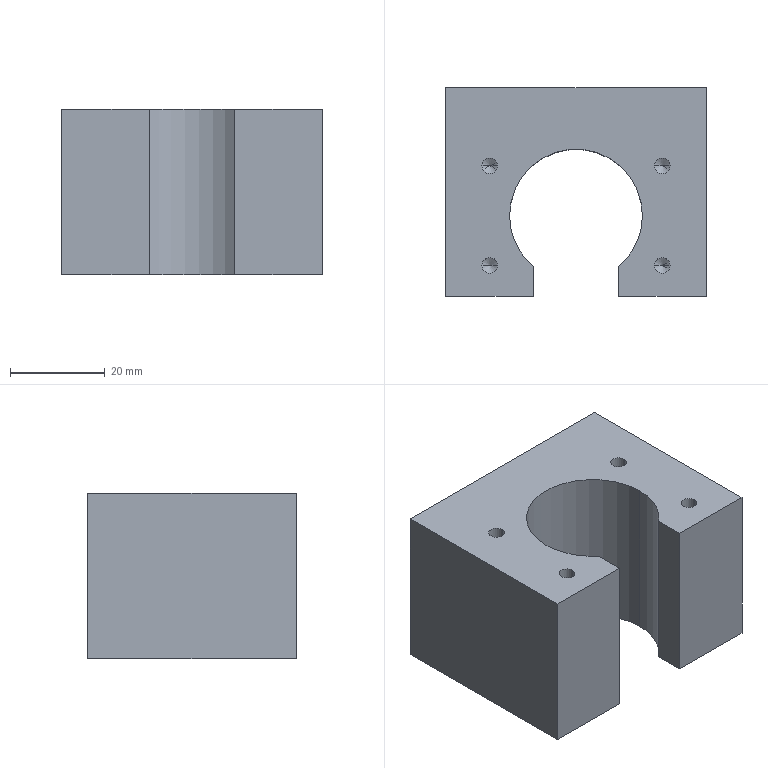Part | SolidWorks | features HoleWzd 2, 3DProfileFeature 1, Extrusion 1 | 1 solid | 52 faces | box 55 x 44 x 35 mm | volume 59279 mm3 | cone 24 | cylinder 19 | plane 9 | commonest cylinder face diameters 3.3 x8 5 x8 28 x3
STEP:
#1=CARTESIAN_POINT('',(-20.5,26.475,8.));
#2=VERTEX_POINT('',#1);
#3=CARTESIAN_POINT('',(-20.5,26.475,13.));
#4=VERTEX_POINT('',#3);
#5=CARTESIAN_POINT('',(-20.5,26.475,10.5));
#6=DIRECTION('',(0.,1.,0.));
#7=DIRECTION('',(0.,0.,1.));
#8=AXIS2_PLACEMENT_3D('',#5,#6,#7);
#9=CIRCLE('',#8,2.5);
#10=EDGE_CURVE('',#2,#4,#9,.T.);
#11=ORIENTED_EDGE('',*,*,#10,.F.);
#12=CARTESIAN_POINT('',(-20.5,27.,7.475));
#13=VERTEX_POINT('',#12);
#14=CARTESIAN_POINT('',(-20.5,27.,7.475));
#15=DIRECTION('',(0.,0.7071,-0.7071));
#16=VECTOR('',#15,1000.);
#17=LINE('',#14,#16);
#18=EDGE_CURVE('',#2,#13,#17,.T.);
#19=ORIENTED_EDGE('',*,*,#18,.T.);
#20=CARTESIAN_POINT('',(-20.5,27.,13.525));
#21=VERTEX_POINT('',#20);
#22=CARTESIAN_POINT('',(-20.5,27.,10.5));
#23=DIRECTION('',(0.,1.,0.));
#24=DIRECTION('',(0.,0.,1.));
#25=AXIS2_PLACEMENT_3D('',#22,#23,#24);
#26=CIRCLE('',#25,3.025);
#27=EDGE_CURVE('',#13,#21,#26,.T.);
#28=ORIENTED_EDGE('',*,*,#27,.T.);
#29=CARTESIAN_POINT('',(-20.5,27.,13.525));
#30=DIRECTION('',(0.,0.7071,0.7071));
#31=VECTOR('',#30,1000.);
#32=LINE('',#29,#31);
#33=EDGE_CURVE('',#4,#21,#32,.T.);
#34=ORIENTED_EDGE('',*,*,#33,.F.);
#35=EDGE_LOOP('',(#11,#19,#28,#34));
#36=FACE_OUTER_BOUND('',#35,.T.);
#37=CARTESIAN_POINT('',(-20.5,27.,10.5));
#38=DIRECTION('',(0.,1.,0.));
#39=DIRECTION('',(0.,0.,1.));
#40=AXIS2_PLACEMENT_3D('',#37,#38,#39);
#41=CONICAL_SURFACE('',#40,3.025,0.7854);
#42=ADVANCED_FACE('',(#36),#41,.F.);
#43=CARTESIAN_POINT('',(-20.5,15.,8.));
#44=VERTEX_POINT('',#43);
#45=CARTESIAN_POINT('',(-20.5,15.,13.));
#46=VERTEX_POINT('',#45);
#47=CARTESIAN_POINT('',(-20.5,15.,10.5));
#48=DIRECTION('',(0.,1.,0.));
#49=DIRECTION('',(0.,0.,1.));
#50=AXIS2_PLACEMENT_3D('',#47,#48,#49);
#51=CIRCLE('',#50,2.5);
#52=EDGE_CURVE('',#44,#46,#51,.T.);
#53=ORIENTED_EDGE('',*,*,#52,.F.);
#54=CARTESIAN_POINT('',(-20.5,27.,8.));
#55=DIRECTION('',(0.,1.,0.));
#56=VECTOR('',#55,1000.);
#57=LINE('',#54,#56);
#58=EDGE_CURVE('',#44,#2,#57,.T.);
#59=ORIENTED_EDGE('',*,*,#58,.T.);
#60=ORIENTED_EDGE('',*,*,#10,.T.);
#61=CARTESIAN_POINT('',(-20.5,27.,13.));
#62=DIRECTION('',(0.,1.,0.));
#63=VECTOR('',#62,1000.);
#64=LINE('',#61,#63);
#65=EDGE_CURVE('',#46,#4,#64,.T.);
#66=ORIENTED_EDGE('',*,*,#65,.F.);
#67=EDGE_LOOP('',(#53,#59,#60,#66));
#68=FACE_OUTER_BOUND('',#67,.T.);
#69=CARTESIAN_POINT('',(-20.5,27.,10.5));
#70=DIRECTION('',(0.,1.,0.));
#71=DIRECTION('',(0.,0.,1.));
#72=AXIS2_PLACEMENT_3D('',#69,#70,#71);
#73=CYLINDRICAL_SURFACE('',#72,2.5);
#74=ADVANCED_FACE('',(#68),#73,.F.);
#75=CARTESIAN_POINT('',(-20.5,13.498,10.5));
#76=VERTEX_POINT('',#75);
#77=CARTESIAN_POINT('',(-20.5,15.,13.));
#78=DIRECTION('',(0.,0.515,0.8572));
#79=VECTOR('',#78,1000.);
#80=LINE('',#77,#79);
#81=EDGE_CURVE('',#76,#46,#80,.T.);
#82=ORIENTED_EDGE('',*,*,#81,.F.);
#83=CARTESIAN_POINT('',(-20.5,15.,8.));
#84=DIRECTION('',(0.,0.515,-0.8572));
#85=VECTOR('',#84,1000.);
#86=LINE('',#83,#85);
#87=EDGE_CURVE('',#76,#44,#86,.T.);
#88=ORIENTED_EDGE('',*,*,#87,.T.);
#89=ORIENTED_EDGE('',*,*,#52,.T.);
#90=EDGE_LOOP('',(#82,#88,#89));
#91=FACE_OUTER_BOUND('',#90,.T.);
#92=CARTESIAN_POINT('',(-20.5,15.,10.5));
#93=DIRECTION('',(0.,1.,0.));
#94=DIRECTION('',(0.,0.,1.));
#95=AXIS2_PLACEMENT_3D('',#92,#93,#94);
#96=CONICAL_SURFACE('',#95,2.5,1.03);
#97=ADVANCED_FACE('',(#91),#96,.F.);
#98=CARTESIAN_POINT('',(-20.5,26.475,-13.));
#99=VERTEX_POINT('',#98);
#100=CARTESIAN_POINT('',(-20.5,26.475,-8.));
#101=VERTEX_POINT('',#100);
#102=CARTESIAN_POINT('',(-20.5,26.475,-10.5));
#103=DIRECTION('',(0.,1.,0.));
#104=DIRECTION('',(0.,0.,1.));
#105=AXIS2_PLACEMENT_3D('',#102,#103,#104);
#106=CIRCLE('',#105,2.5);
#107=EDGE_CURVE('',#99,#101,#106,.T.);
#108=ORIENTED_EDGE('',*,*,#107,.F.);
#109=CARTESIAN_POINT('',(-20.5,27.,-13.525));
#110=VERTEX_POINT('',#109);
#111=CARTESIAN_POINT('',(-20.5,27.,-13.525));
#112=DIRECTION('',(0.,0.7071,-0.7071));
#113=VECTOR('',#112,1000.);
#114=LINE('',#111,#113);
#115=EDGE_CURVE('',#99,#110,#114,.T.);
#116=ORIENTED_EDGE('',*,*,#115,.T.);
#117=CARTESIAN_POINT('',(-20.5,27.,-7.475));
#118=VERTEX_POINT('',#117);
#119=CARTESIAN_POINT('',(-20.5,27.,-10.5));
#120=DIRECTION('',(0.,1.,0.));
#121=DIRECTION('',(0.,0.,1.));
#122=AXIS2_PLACEMENT_3D('',#119,#120,#121);
#123=CIRCLE('',#122,3.025);
#124=EDGE_CURVE('',#110,#118,#123,.T.);
#125=ORIENTED_EDGE('',*,*,#124,.T.);
#126=CARTESIAN_POINT('',(-20.5,27.,-7.475));
#127=DIRECTION('',(0.,0.7071,0.7071));
#128=VECTOR('',#127,1000.);
#129=LINE('',#126,#128);
#130=EDGE_CURVE('',#101,#118,#129,.T.);
#131=ORIENTED_EDGE('',*,*,#130,.F.);
#132=EDGE_LOOP('',(#108,#116,#125,#131));
#133=FACE_OUTER_BOUND('',#132,.T.);
#134=CARTESIAN_POINT('',(-20.5,27.,-10.5));
#135=DIRECTION('',(0.,1.,0.));
#136=DIRECTION('',(0.,0.,1.));
#137=AXIS2_PLACEMENT_3D('',#134,#135,#136);
#138=CONICAL_SURFACE('',#137,3.025,0.7854);
#139=ADVANCED_FACE('',(#133),#138,.F.);
#140=CARTESIAN_POINT('',(-20.5,15.,-13.));
#141=VERTEX_POINT('',#140);
#142=CARTESIAN_POINT('',(-20.5,15.,-8.));
#143=VERTEX_POINT('',#142);
#144=CARTESIAN_POINT('',(-20.5,15.,-10.5));
#145=DIRECTION('',(0.,1.,0.));
#146=DIRECTION('',(0.,0.,1.));
#147=AXIS2_PLACEMENT_3D('',#144,#145,#146);
#148=CIRCLE('',#147,2.5);
#149=EDGE_CURVE('',#141,#143,#148,.T.);
#150=ORIENTED_EDGE('',*,*,#149,.F.);
#151=CARTESIAN_POINT('',(-20.5,27.,-13.));
#152=DIRECTION('',(0.,1.,0.));
#153=VECTOR('',#152,1000.);
#154=LINE('',#151,#153);
#155=EDGE_CURVE('',#141,#99,#154,.T.);
#156=ORIENTED_EDGE('',*,*,#155,.T.);
#157=ORIENTED_EDGE('',*,*,#107,.T.);
#158=CARTESIAN_POINT('',(-20.5,27.,-8.));
#159=DIRECTION('',(0.,1.,0.));
#160=VECTOR('',#159,1000.);
#161=LINE('',#158,#160);
#162=EDGE_CURVE('',#143,#101,#161,.T.);
#163=ORIENTED_EDGE('',*,*,#162,.F.);
#164=EDGE_LOOP('',(#150,#156,#157,#163));
#165=FACE_OUTER_BOUND('',#164,.T.);
#166=CARTESIAN_POINT('',(-20.5,27.,-10.5));
#167=DIRECTION('',(0.,1.,0.));
#168=DIRECTION('',(0.,0.,1.));
#169=AXIS2_PLACEMENT_3D('',#166,#167,#168);
#170=CYLINDRICAL_SURFACE('',#169,2.5);
#171=ADVANCED_FACE('',(#165),#170,.F.);
#172=CARTESIAN_POINT('',(-20.5,13.498,-10.5));
#173=VERTEX_POINT('',#172);
#174=CARTESIAN_POINT('',(-20.5,15.,-8.));
#175=DIRECTION('',(0.,0.515,0.8572));
#176=VECTOR('',#175,1000.);
#177=LINE('',#174,#176);
#178=EDGE_CURVE('',#173,#143,#177,.T.);
#179=ORIENTED_EDGE('',*,*,#178,.F.);
#180=CARTESIAN_POINT('',(-20.5,15.,-13.));
#181=DIRECTION('',(0.,0.515,-0.8572));
#182=VECTOR('',#181,1000.);
#183=LINE('',#180,#182);
#184=EDGE_CURVE('',#173,#141,#183,.T.);
#185=ORIENTED_EDGE('',*,*,#184,.T.);
#186=ORIENTED_EDGE('',*,*,#149,.T.);
#187=EDGE_LOOP('',(#179,#185,#186));
#188=FACE_OUTER_BOUND('',#187,.T.);
#189=CARTESIAN_POINT('',(-20.5,15.,-10.5));
#190=DIRECTION('',(0.,1.,0.));
#191=DIRECTION('',(0.,0.,1.));
#192=AXIS2_PLACEMENT_3D('',#189,#190,#191);
#193=CONICAL_SURFACE('',#192,2.5,1.03);
#194=ADVANCED_FACE('',(#188),#193,.F.);
#195=CARTESIAN_POINT('',(20.5,26.475,-13.));
#196=VERTEX_POINT('',#195);
#197=CARTESIAN_POINT('',(20.5,26.475,-8.));
#198=VERTEX_POINT('',#197);
#199=CARTESIAN_POINT('',(20.5,26.475,-10.5));
#200=DIRECTION('',(0.,1.,0.));
#201=DIRECTION('',(0.,0.,1.));
#202=AXIS2_PLACEMENT_3D('',#199,#200,#201);
#203=CIRCLE('',#202,2.5);
#204=EDGE_CURVE('',#196,#198,#203,.T.);
#205=ORIENTED_EDGE('',*,*,#204,.F.);
#206=CARTESIAN_POINT('',(20.5,27.,-13.525));
#207=VERTEX_POINT('',#206);
#208=CARTESIAN_POINT('',(20.5,27.,-13.525));
#209=DIRECTION('',(0.,0.7071,-0.7071));
#210=VECTOR('',#209,1000.);
#211=LINE('',#208,#210);
#212=EDGE_CURVE('',#196,#207,#211,.T.);
#213=ORIENTED_EDGE('',*,*,#212,.T.);
#214=CARTESIAN_POINT('',(20.5,27.,-7.475));
#215=VERTEX_POINT('',#214);
#216=CARTESIAN_POINT('',(20.5,27.,-10.5));
#217=DIRECTION('',(0.,1.,0.));
#218=DIRECTION('',(0.,0.,1.));
#219=AXIS2_PLACEMENT_3D('',#216,#217,#218);
#220=CIRCLE('',#219,3.025);
#221=EDGE_CURVE('',#207,#215,#220,.T.);
#222=ORIENTED_EDGE('',*,*,#221,.T.);
#223=CARTESIAN_POINT('',(20.5,27.,-7.475));
#224=DIRECTION('',(0.,0.7071,0.7071));
#225=VECTOR('',#224,1000.);
#226=LINE('',#223,#225);
#227=EDGE_CURVE('',#198,#215,#226,.T.);
#228=ORIENTED_EDGE('',*,*,#227,.F.);
#229=EDGE_LOOP('',(#205,#213,#222,#228));
#230=FACE_OUTER_BOUND('',#229,.T.);
#231=CARTESIAN_POINT('',(20.5,27.,-10.5));
#232=DIRECTION('',(0.,1.,0.));
#233=DIRECTION('',(0.,0.,1.));
#234=AXIS2_PLACEMENT_3D('',#231,#232,#233);
#235=CONICAL_SURFACE('',#234,3.025,0.7854);
#236=ADVANCED_FACE('',(#230),#235,.F.);
#237=CARTESIAN_POINT('',(20.5,15.,-13.));
#238=VERTEX_POINT('',#237);
#239=CARTESIAN_POINT('',(20.5,15.,-8.));
#240=VERTEX_POINT('',#239);
#241=CARTESIAN_POINT('',(20.5,15.,-10.5));
#242=DIRECTION('',(0.,1.,0.));
#243=DIRECTION('',(0.,0.,1.));
#244=AXIS2_PLACEMENT_3D('',#241,#242,#243);
#245=CIRCLE('',#244,2.5);
#246=EDGE_CURVE('',#238,#240,#245,.T.);
#247=ORIENTED_EDGE('',*,*,#246,.F.);
#248=CARTESIAN_POINT('',(20.5,27.,-13.));
#249=DIRECTION('',(0.,1.,0.));
#250=VECTOR('',#249,1000.);
#251=LINE('',#248,#250);
#252=EDGE_CURVE('',#238,#196,#251,.T.);
#253=ORIENTED_EDGE('',*,*,#252,.T.);
#254=ORIENTED_EDGE('',*,*,#204,.T.);
#255=CARTESIAN_POINT('',(20.5,27.,-8.));
#256=DIRECTION('',(0.,1.,0.));
#257=VECTOR('',#256,1000.);
#258=LINE('',#255,#257);
#259=EDGE_CURVE('',#240,#198,#258,.T.);
#260=ORIENTED_EDGE('',*,*,#259,.F.);
#261=EDGE_LOOP('',(#247,#253,#254,#260));
#262=FACE_OUTER_BOUND('',#261,.T.);
#263=CARTESIAN_POINT('',(20.5,27.,-10.5));
#264=DIRECTION('',(0.,1.,0.));
#265=DIRECTION('',(0.,0.,1.));
#266=AXIS2_PLACEMENT_3D('',#263,#264,#265);
#267=CYLINDRICAL_SURFACE('',#266,2.5);
#268=ADVANCED_FACE('',(#262),#267,.F.);
#269=CARTESIAN_POINT('',(20.5,13.498,-10.5));
#270=VERTEX_POINT('',#269);
#271=CARTESIAN_POINT('',(20.5,15.,-8.));
#272=DIRECTION('',(0.,0.515,0.8572));
#273=VECTOR('',#272,1000.);
#274=LINE('',#271,#273);
#275=EDGE_CURVE('',#270,#240,#274,.T.);
#276=ORIENTED_EDGE('',*,*,#275,.F.);
#277=CARTESIAN_POINT('',(20.5,15.,-13.));
#278=DIRECTION('',(0.,0.515,-0.8572));
#279=VECTOR('',#278,1000.);
#280=LINE('',#277,#279);
#281=EDGE_CURVE('',#270,#238,#280,.T.);
#282=ORIENTED_EDGE('',*,*,#281,.T.);
#283=ORIENTED_EDGE('',*,*,#246,.T.);
#284=EDGE_LOOP('',(#276,#282,#283));
#285=FACE_OUTER_BOUND('',#284,.T.);
#286=CARTESIAN_POINT('',(20.5,15.,-10.5));
#287=DIRECTION('',(0.,1.,0.));
#288=DIRECTION('',(0.,0.,1.));
#289=AXIS2_PLACEMENT_3D('',#286,#287,#288);
#290=CONICAL_SURFACE('',#289,2.5,1.03);
#291=ADVANCED_FACE('',(#285),#290,.F.);
#292=CARTESIAN_POINT('',(20.5,26.475,8.));
#293=VERTEX_POINT('',#292);
#294=CARTESIAN_POINT('',(20.5,26.475,13.));
#295=VERTEX_POINT('',#294);
#296=CARTESIAN_POINT('',(20.5,26.475,10.5));
#297=DIRECTION('',(0.,1.,0.));
#298=DIRECTION('',(0.,0.,1.));
#299=AXIS2_PLACEMENT_3D('',#296,#297,#298);
#300=CIRCLE('',#299,2.5);
#301=EDGE_CURVE('',#293,#295,#300,.T.);
#302=ORIENTED_EDGE('',*,*,#301,.F.);
#303=CARTESIAN_POINT('',(20.5,27.,7.475));
#304=VERTEX_POINT('',#303);
#305=CARTESIAN_POINT('',(20.5,27.,7.475));
#306=DIRECTION('',(0.,0.7071,-0.7071));
#307=VECTOR('',#306,1000.);
#308=LINE('',#305,#307);
#309=EDGE_CURVE('',#293,#304,#308,.T.);
#310=ORIENTED_EDGE('',*,*,#309,.T.);
#311=CARTESIAN_POINT('',(20.5,27.,13.525));
#312=VERTEX_POINT('',#311);
#313=CARTESIAN_POINT('',(20.5,27.,10.5));
#314=DIRECTION('',(0.,1.,0.));
#315=DIRECTION('',(0.,0.,1.));
#316=AXIS2_PLACEMENT_3D('',#313,#314,#315);
#317=CIRCLE('',#316,3.025);
#318=EDGE_CURVE('',#304,#312,#317,.T.);
#319=ORIENTED_EDGE('',*,*,#318,.T.);
#320=CARTESIAN_POINT('',(20.5,27.,13.525));
#321=DIRECTION('',(0.,0.7071,0.7071));
#322=VECTOR('',#321,1000.);
#323=LINE('',#320,#322);
#324=EDGE_CURVE('',#295,#312,#323,.T.);
#325=ORIENTED_EDGE('',*,*,#324,.F.);
#326=EDGE_LOOP('',(#302,#310,#319,#325));
#327=FACE_OUTER_BOUND('',#326,.T.);
#328=CARTESIAN_POINT('',(20.5,27.,10.5));
#329=DIRECTION('',(0.,1.,0.));
#330=DIRECTION('',(0.,0.,1.));
#331=AXIS2_PLACEMENT_3D('',#328,#329,#330);
#332=CONICAL_SURFACE('',#331,3.025,0.7854);
#333=ADVANCED_FACE('',(#327),#332,.F.);
#334=CARTESIAN_POINT('',(20.5,15.,8.));
#335=VERTEX_POINT('',#334);
#336=CARTESIAN_POINT('',(20.5,15.,13.));
#337=VERTEX_POINT('',#336);
#338=CARTESIAN_POINT('',(20.5,15.,10.5));
#339=DIRECTION('',(0.,1.,0.));
#340=DIRECTION('',(0.,0.,1.));
#341=AXIS2_PLACEMENT_3D('',#338,#339,#340);
#342=CIRCLE('',#341,2.5);
#343=EDGE_CURVE('',#335,#337,#342,.T.);
#344=ORIENTED_EDGE('',*,*,#343,.F.);
#345=CARTESIAN_POINT('',(20.5,27.,8.));
#346=DIRECTION('',(0.,1.,0.));
#347=VECTOR('',#346,1000.);
#348=LINE('',#345,#347);
#349=EDGE_CURVE('',#335,#293,#348,.T.);
#350=ORIENTED_EDGE('',*,*,#349,.T.);
#351=ORIENTED_EDGE('',*,*,#301,.T.);
#352=CARTESIAN_POINT('',(20.5,27.,13.));
#353=DIRECTION('',(0.,1.,0.));
#354=VECTOR('',#353,1000.);
#355=LINE('',#352,#354);
#356=EDGE_CURVE('',#337,#295,#355,.T.);
#357=ORIENTED_EDGE('',*,*,#356,.F.);
#358=EDGE_LOOP('',(#344,#350,#351,#357));
#359=FACE_OUTER_BOUND('',#358,.T.);
#360=CARTESIAN_POINT('',(20.5,27.,10.5));
#361=DIRECTION('',(0.,1.,0.));
#362=DIRECTION('',(0.,0.,1.));
#363=AXIS2_PLACEMENT_3D('',#360,#361,#362);
#364=CYLINDRICAL_SURFACE('',#363,2.5);
#365=ADVANCED_FACE('',(#359),#364,.F.);
#366=CARTESIAN_POINT('',(20.5,13.498,10.5));
#367=VERTEX_POINT('',#366);
#368=CARTESIAN_POINT('',(20.5,15.,13.));
#369=DIRECTION('',(0.,0.515,0.8572));
#370=VECTOR('',#369,1000.);
#371=LINE('',#368,#370);
#372=EDGE_CURVE('',#367,#337,#371,.T.);
#373=ORIENTED_EDGE('',*,*,#372,.F.);
#374=CARTESIAN_POINT('',(20.5,15.,8.));
#375=DIRECTION('',(0.,0.515,-0.8572));
#376=VECTOR('',#375,1000.);
#377=LINE('',#374,#376);
#378=EDGE_CURVE('',#367,#335,#377,.T.);
#379=ORIENTED_EDGE('',*,*,#378,.T.);
#380=ORIENTED_EDGE('',*,*,#343,.T.);
#381=EDGE_LOOP('',(#373,#379,#380));
#382=FACE_OUTER_BOUND('',#381,.T.);
#383=CARTESIAN_POINT('',(20.5,15.,10.5));
#384=DIRECTION('',(0.,1.,0.));
#385=DIRECTION('',(0.,0.,1.));
#386=AXIS2_PLACEMENT_3D('',#383,#384,#385);
#387=CONICAL_SURFACE('',#386,2.5,1.03);
#388=ADVANCED_FACE('',(#382),#387,.F.);
#389=CARTESIAN_POINT('',(16.537,10.5,8.));
#390=VERTEX_POINT('',#389);
#391=CARTESIAN_POINT('',(19.837,10.5,8.));
#392=VERTEX_POINT('',#391);
#393=CARTESIAN_POINT('',(18.187,10.5,8.));
#394=DIRECTION('',(0.,0.,1.));
#395=DIRECTION('',(1.,0.,0.));
#396=AXIS2_PLACEMENT_3D('',#393,#394,#395);
#397=CIRCLE('',#396,1.65);
#398=EDGE_CURVE('',#390,#392,#397,.T.);
#399=ORIENTED_EDGE('',*,*,#398,.F.);
#400=CARTESIAN_POINT('',(16.537,10.5,17.5));
#401=VERTEX_POINT('',#400);
#402=CARTESIAN_POINT('',(16.537,10.5,17.5));
#403=DIRECTION('',(0.,0.,1.));
#404=VECTOR('',#403,1000.);
#405=LINE('',#402,#404);
#406=EDGE_CURVE('',#390,#401,#405,.T.);
#407=ORIENTED_EDGE('',*,*,#406,.T.);
#408=CARTESIAN_POINT('',(19.837,10.5,17.5));
#409=VERTEX_POINT('',#408);
#410=CARTESIAN_POINT('',(18.187,10.5,17.5));
#411=DIRECTION('',(0.,0.,1.));
#412=DIRECTION('',(1.,0.,0.));
#413=AXIS2_PLACEMENT_3D('',#410,#411,#412);
#414=CIRCLE('',#413,1.65);
#415=EDGE_CURVE('',#401,#409,#414,.T.);
#416=ORIENTED_EDGE('',*,*,#415,.T.);
#417=CARTESIAN_POINT('',(19.837,10.5,17.5));
#418=DIRECTION('',(0.,0.,1.));
#419=VECTOR('',#418,1000.);
#420=LINE('',#417,#419);
#421=EDGE_CURVE('',#392,#409,#420,.T.);
#422=ORIENTED_EDGE('',*,*,#421,.F.);
#423=EDGE_LOOP('',(#399,#407,#416,#422));
#424=FACE_OUTER_BOUND('',#423,.T.);
#425=CARTESIAN_POINT('',(18.187,10.5,17.5));
#426=DIRECTION('',(0.,0.,1.));
#427=DIRECTION('',(1.,0.,0.));
#428=AXIS2_PLACEMENT_3D('',#425,#426,#427);
#429=CYLINDRICAL_SURFACE('',#428,1.65);
#430=ADVANCED_FACE('',(#424),#429,.F.);
#431=CARTESIAN_POINT('',(18.187,10.5,7.009));
#432=VERTEX_POINT('',#431);
#433=CARTESIAN_POINT('',(19.837,10.5,8.));
#434=DIRECTION('',(0.8572,0.,0.515));
#435=VECTOR('',#434,1000.);
#436=LINE('',#433,#435);
#437=EDGE_CURVE('',#432,#392,#436,.T.);
#438=ORIENTED_EDGE('',*,*,#437,.F.);
#439=CARTESIAN_POINT('',(16.537,10.5,8.));
#440=DIRECTION('',(-0.8572,0.,0.515));
#441=VECTOR('',#440,1000.);
#442=LINE('',#439,#441);
#443=EDGE_CURVE('',#432,#390,#442,.T.);
#444=ORIENTED_EDGE('',*,*,#443,.T.);
#445=ORIENTED_EDGE('',*,*,#398,.T.);
#446=EDGE_LOOP('',(#438,#444,#445));
#447=FACE_OUTER_BOUND('',#446,.T.);
#448=CARTESIAN_POINT('',(18.187,10.5,8.));
#449=DIRECTION('',(0.,0.,1.));
#450=DIRECTION('',(1.,0.,0.));
#451=AXIS2_PLACEMENT_3D('',#448,#449,#450);
#452=CONICAL_SURFACE('',#451,1.65,1.03);
#453=ADVANCED_FACE('',(#447),#452,.F.);
#454=CARTESIAN_POINT('',(16.537,-10.5,8.));
#455=VERTEX_POINT('',#454);
#456=CARTESIAN_POINT('',(19.837,-10.5,8.));
#457=VERTEX_POINT('',#456);
#458=CARTESIAN_POINT('',(18.187,-10.5,8.));
#459=DIRECTION('',(0.,0.,1.));
#460=DIRECTION('',(1.,0.,0.));
#461=AXIS2_PLACEMENT_3D('',#458,#459,#460);
#462=CIRCLE('',#461,1.65);
#463=EDGE_CURVE('',#455,#457,#462,.T.);
#464=ORIENTED_EDGE('',*,*,#463,.F.);
#465=CARTESIAN_POINT('',(16.537,-10.5,17.5));
#466=VERTEX_POINT('',#465);
#467=CARTESIAN_POINT('',(16.537,-10.5,17.5));
#468=DIRECTION('',(0.,0.,1.));
#469=VECTOR('',#468,1000.);
#470=LINE('',#467,#469);
#471=EDGE_CURVE('',#455,#466,#470,.T.);
#472=ORIENTED_EDGE('',*,*,#471,.T.);
#473=CARTESIAN_POINT('',(19.837,-10.5,17.5));
#474=VERTEX_POINT('',#473);
#475=CARTESIAN_POINT('',(18.187,-10.5,17.5));
#476=DIRECTION('',(0.,0.,1.));
#477=DIRECTION('',(1.,0.,0.));
#478=AXIS2_PLACEMENT_3D('',#475,#476,#477);
#479=CIRCLE('',#478,1.65);
#480=EDGE_CURVE('',#466,#474,#479,.T.);
#481=ORIENTED_EDGE('',*,*,#480,.T.);
#482=CARTESIAN_POINT('',(19.837,-10.5,17.5));
#483=DIRECTION('',(0.,0.,1.));
#484=VECTOR('',#483,1000.);
#485=LINE('',#482,#484);
#486=EDGE_CURVE('',#457,#474,#485,.T.);
#487=ORIENTED_EDGE('',*,*,#486,.F.);
#488=EDGE_LOOP('',(#464,#472,#481,#487));
#489=FACE_OUTER_BOUND('',#488,.T.);
#490=CARTESIAN_POINT('',(18.187,-10.5,17.5));
#491=DIRECTION('',(0.,0.,1.));
#492=DIRECTION('',(1.,0.,0.));
#493=AXIS2_PLACEMENT_3D('',#490,#491,#492);
#494=CYLINDRICAL_SURFACE('',#493,1.65);
#495=ADVANCED_FACE('',(#489),#494,.F.);
#496=CARTESIAN_POINT('',(18.187,-10.5,7.009));
#497=VERTEX_POINT('',#496);
#498=CARTESIAN_POINT('',(19.837,-10.5,8.));
#499=DIRECTION('',(0.8572,0.,0.515));
#500=VECTOR('',#499,1000.);
#501=LINE('',#498,#500);
#502=EDGE_CURVE('',#497,#457,#501,.T.);
#503=ORIENTED_EDGE('',*,*,#502,.F.);
#504=CARTESIAN_POINT('',(16.537,-10.5,8.));
#505=DIRECTION('',(-0.8572,0.,0.515));
#506=VECTOR('',#505,1000.);
#507=LINE('',#504,#506);
#508=EDGE_CURVE('',#497,#455,#507,.T.);
#509=ORIENTED_EDGE('',*,*,#508,.T.);
#510=ORIENTED_EDGE('',*,*,#463,.T.);
#511=EDGE_LOOP('',(#503,#509,#510));
#512=FACE_OUTER_BOUND('',#511,.T.);
#513=CARTESIAN_POINT('',(18.187,-10.5,8.));
#514=DIRECTION('',(0.,0.,1.));
#515=DIRECTION('',(1.,0.,0.));
#516=AXIS2_PLACEMENT_3D('',#513,#514,#515);
#517=CONICAL_SURFACE('',#516,1.65,1.03);
#518=ADVANCED_FACE('',(#512),#517,.F.);
#519=CARTESIAN_POINT('',(-19.837,-10.5,8.));
#520=VERTEX_POINT('',#519);
#521=CARTESIAN_POINT('',(-16.537,-10.5,8.));
#522=VERTEX_POINT('',#521);
#523=CARTESIAN_POINT('',(-18.187,-10.5,8.));
#524=DIRECTION('',(0.,0.,1.));
#525=DIRECTION('',(1.,0.,0.));
#526=AXIS2_PLACEMENT_3D('',#523,#524,#525);
#527=CIRCLE('',#526,1.65);
#528=EDGE_CURVE('',#520,#522,#527,.T.);
#529=ORIENTED_EDGE('',*,*,#528,.F.);
#530=CARTESIAN_POINT('',(-19.837,-10.5,17.5));
#531=VERTEX_POINT('',#530);
#532=CARTESIAN_POINT('',(-19.837,-10.5,17.5));
#533=DIRECTION('',(0.,0.,1.));
#534=VECTOR('',#533,1000.);
#535=LINE('',#532,#534);
#536=EDGE_CURVE('',#520,#531,#535,.T.);
#537=ORIENTED_EDGE('',*,*,#536,.T.);
#538=CARTESIAN_POINT('',(-16.537,-10.5,17.5));
#539=VERTEX_POINT('',#538);
#540=CARTESIAN_POINT('',(-18.187,-10.5,17.5));
#541=DIRECTION('',(0.,0.,1.));
#542=DIRECTION('',(1.,0.,0.));
#543=AXIS2_PLACEMENT_3D('',#540,#541,#542);
#544=CIRCLE('',#543,1.65);
#545=EDGE_CURVE('',#531,#539,#544,.T.);
#546=ORIENTED_EDGE('',*,*,#545,.T.);
#547=CARTESIAN_POINT('',(-16.537,-10.5,17.5));
#548=DIRECTION('',(0.,0.,1.));
#549=VECTOR('',#548,1000.);
#550=LINE('',#547,#549);
#551=EDGE_CURVE('',#522,#539,#550,.T.);
#552=ORIENTED_EDGE('',*,*,#551,.F.);
#553=EDGE_LOOP('',(#529,#537,#546,#552));
#554=FACE_OUTER_BOUND('',#553,.T.);
#555=CARTESIAN_POINT('',(-18.187,-10.5,17.5));
#556=DIRECTION('',(0.,0.,1.));
#557=DIRECTION('',(1.,0.,0.));
#558=AXIS2_PLACEMENT_3D('',#555,#556,#557);
#559=CYLINDRICAL_SURFACE('',#558,1.65);
#560=ADVANCED_FACE('',(#554),#559,.F.);
#561=CARTESIAN_POINT('',(-18.187,-10.5,7.009));
#562=VERTEX_POINT('',#561);
#563=CARTESIAN_POINT('',(-16.537,-10.5,8.));
#564=DIRECTION('',(0.8572,0.,0.515));
#565=VECTOR('',#564,1000.);
#566=LINE('',#563,#565);
#567=EDGE_CURVE('',#562,#522,#566,.T.);
#568=ORIENTED_EDGE('',*,*,#567,.F.);
#569=CARTESIAN_POINT('',(-19.837,-10.5,8.));
#570=DIRECTION('',(-0.8572,0.,0.515));
#571=VECTOR('',#570,1000.);
#572=LINE('',#569,#571);
#573=EDGE_CURVE('',#562,#520,#572,.T.);
#574=ORIENTED_EDGE('',*,*,#573,.T.);
#575=ORIENTED_EDGE('',*,*,#528,.T.);
#576=EDGE_LOOP('',(#568,#574,#575));
#577=FACE_OUTER_BOUND('',#576,.T.);
#578=CARTESIAN_POINT('',(-18.187,-10.5,8.));
#579=DIRECTION('',(0.,0.,1.));
#580=DIRECTION('',(1.,0.,0.));
#581=AXIS2_PLACEMENT_3D('',#578,#579,#580);
#582=CONICAL_SURFACE('',#581,1.65,1.03);
#583=ADVANCED_FACE('',(#577),#582,.F.);
#584=CARTESIAN_POINT('',(-19.837,10.5,8.));
#585=VERTEX_POINT('',#584);
#586=CARTESIAN_POINT('',(-16.537,10.5,8.));
#587=VERTEX_POINT('',#586);
#588=CARTESIAN_POINT('',(-18.187,10.5,8.));
#589=DIRECTION('',(0.,0.,1.));
#590=DIRECTION('',(1.,0.,0.));
#591=AXIS2_PLACEMENT_3D('',#588,#589,#590);
#592=CIRCLE('',#591,1.65);
#593=EDGE_CURVE('',#585,#587,#592,.T.);
#594=ORIENTED_EDGE('',*,*,#593,.F.);
#595=CARTESIAN_POINT('',(-19.837,10.5,17.5));
#596=VERTEX_POINT('',#595);
#597=CARTESIAN_POINT('',(-19.837,10.5,17.5));
#598=DIRECTION('',(0.,0.,1.));
#599=VECTOR('',#598,1000.);
#600=LINE('',#597,#599);
#601=EDGE_CURVE('',#585,#596,#600,.T.);
#602=ORIENTED_EDGE('',*,*,#601,.T.);
#603=CARTESIAN_POINT('',(-16.537,10.5,17.5));
#604=VERTEX_POINT('',#603);
#605=CARTESIAN_POINT('',(-18.187,10.5,17.5));
#606=DIRECTION('',(0.,0.,1.));
#607=DIRECTION('',(1.,0.,0.));
#608=AXIS2_PLACEMENT_3D('',#605,#606,#607);
#609=CIRCLE('',#608,1.65);
#610=EDGE_CURVE('',#596,#604,#609,.T.);
#611=ORIENTED_EDGE('',*,*,#610,.T.);
#612=CARTESIAN_POINT('',(-16.537,10.5,17.5));
#613=DIRECTION('',(0.,0.,1.));
#614=VECTOR('',#613,1000.);
#615=LINE('',#612,#614);
#616=EDGE_CURVE('',#587,#604,#615,.T.);
#617=ORIENTED_EDGE('',*,*,#616,.F.);
#618=EDGE_LOOP('',(#594,#602,#611,#617));
#619=FACE_OUTER_BOUND('',#618,.T.);
#620=CARTESIAN_POINT('',(-18.187,10.5,17.5));
#621=DIRECTION('',(0.,0.,1.));
#622=DIRECTION('',(1.,0.,0.));
#623=AXIS2_PLACEMENT_3D('',#620,#621,#622);
#624=CYLINDRICAL_SURFACE('',#623,1.65);
#625=ADVANCED_FACE('',(#619),#624,.F.);
#626=CARTESIAN_POINT('',(-18.187,10.5,7.009));
#627=VERTEX_POINT('',#626);
#628=CARTESIAN_POINT('',(-16.537,10.5,8.));
#629=DIRECTION('',(0.8572,0.,0.515));
#630=VECTOR('',#629,1000.);
#631=LINE('',#628,#630);
#632=EDGE_CURVE('',#627,#587,#631,.T.);
#633=ORIENTED_EDGE('',*,*,#632,.F.);
#634=CARTESIAN_POINT('',(-19.837,10.5,8.));
#635=DIRECTION('',(-0.8572,0.,0.515));
#636=VECTOR('',#635,1000.);
#637=LINE('',#634,#636);
#638=EDGE_CURVE('',#627,#585,#637,.T.);
#639=ORIENTED_EDGE('',*,*,#638,.T.);
#640=ORIENTED_EDGE('',*,*,#593,.T.);
#641=EDGE_LOOP('',(#633,#639,#640));
#642=FACE_OUTER_BOUND('',#641,.T.);
#643=CARTESIAN_POINT('',(-18.187,10.5,8.));
#644=DIRECTION('',(0.,0.,1.));
#645=DIRECTION('',(1.,0.,0.));
#646=AXIS2_PLACEMENT_3D('',#643,#644,#645);
#647=CONICAL_SURFACE('',#646,1.65,1.03);
#648=ADVANCED_FACE('',(#642),#647,.F.);
#649=CARTESIAN_POINT('',(14.,0.,17.5));
#650=VERTEX_POINT('',#649);
#651=CARTESIAN_POINT('',(9.,-10.724,17.5));
#652=VERTEX_POINT('',#651);
#653=CARTESIAN_POINT('',(0.,0.,17.5));
#654=DIRECTION('',(0.,0.,-1.));
#655=DIRECTION('',(1.,0.,0.));
#656=AXIS2_PLACEMENT_3D('',#653,#654,#655);
#657=CIRCLE('',#656,14.);
#658=EDGE_CURVE('',#650,#652,#657,.T.);
#659=ORIENTED_EDGE('',*,*,#658,.F.);
#660=CARTESIAN_POINT('',(14.,0.,-17.5));
#661=VERTEX_POINT('',#660);
#662=CARTESIAN_POINT('',(14.,0.,17.5));
#663=DIRECTION('',(0.,0.,-1.));
#664=VECTOR('',#663,1000.);
#665=LINE('',#662,#664);
#666=EDGE_CURVE('',#650,#661,#665,.T.);
#667=ORIENTED_EDGE('',*,*,#666,.T.);
#668=CARTESIAN_POINT('',(9.,-10.724,-17.5));
#669=VERTEX_POINT('',#668);
#670=CARTESIAN_POINT('',(0.,0.,-17.5));
#671=DIRECTION('',(0.,0.,-1.));
#672=DIRECTION('',(1.,0.,0.));
#673=AXIS2_PLACEMENT_3D('',#670,#671,#672);
#674=CIRCLE('',#673,14.);
#675=EDGE_CURVE('',#661,#669,#674,.T.);
#676=ORIENTED_EDGE('',*,*,#675,.T.);
#677=CARTESIAN_POINT('',(9.,-10.724,17.5));
#678=DIRECTION('',(0.,0.,-1.));
#679=VECTOR('',#678,1000.);
#680=LINE('',#677,#679);
#681=EDGE_CURVE('',#652,#669,#680,.T.);
#682=ORIENTED_EDGE('',*,*,#681,.F.);
#683=EDGE_LOOP('',(#659,#667,#676,#682));
#684=FACE_OUTER_BOUND('',#683,.T.);
#685=CARTESIAN_POINT('',(0.,0.,17.5));
#686=DIRECTION('',(0.,0.,-1.));
#687=DIRECTION('',(-1.,0.,0.));
#688=AXIS2_PLACEMENT_3D('',#685,#686,#687);
#689=CYLINDRICAL_SURFACE('',#688,14.);
#690=ADVANCED_FACE('',(#684),#689,.F.);
#691=ORIENTED_EDGE('',*,*,#666,.F.);
#692=CARTESIAN_POINT('',(-14.,0.,17.5));
#693=VERTEX_POINT('',#692);
#694=CARTESIAN_POINT('',(0.,0.,17.5));
#695=DIRECTION('',(0.,0.,-1.));
#696=DIRECTION('',(1.,0.,0.));
#697=AXIS2_PLACEMENT_3D('',#694,#695,#696);
#698=CIRCLE('',#697,14.);
#699=EDGE_CURVE('',#693,#650,#698,.T.);
#700=ORIENTED_EDGE('',*,*,#699,.F.);
#701=CARTESIAN_POINT('',(-14.,0.,-17.5));
#702=VERTEX_POINT('',#701);
#703=CARTESIAN_POINT('',(-14.,0.,17.5));
#704=DIRECTION('',(0.,0.,-1.));
#705=VECTOR('',#704,1000.);
#706=LINE('',#703,#705);
#707=EDGE_CURVE('',#693,#702,#706,.T.);
#708=ORIENTED_EDGE('',*,*,#707,.T.);
#709=CARTESIAN_POINT('',(0.,0.,-17.5));
#710=DIRECTION('',(0.,0.,-1.));
#711=DIRECTION('',(1.,0.,0.));
#712=AXIS2_PLACEMENT_3D('',#709,#710,#711);
#713=CIRCLE('',#712,14.);
#714=EDGE_CURVE('',#702,#661,#713,.T.);
#715=ORIENTED_EDGE('',*,*,#714,.T.);
#716=EDGE_LOOP('',(#691,#700,#708,#715));
#717=FACE_OUTER_BOUND('',#716,.T.);
#718=CARTESIAN_POINT('',(0.,0.,17.5));
#719=DIRECTION('',(0.,0.,-1.));
#720=DIRECTION('',(-1.,0.,0.));
#721=AXIS2_PLACEMENT_3D('',#718,#719,#720);
#722=CYLINDRICAL_SURFACE('',#721,14.);
#723=ADVANCED_FACE('',(#717),#722,.F.);
#724=CARTESIAN_POINT('',(-27.5,27.,-17.5));
#725=VERTEX_POINT('',#724);
#726=CARTESIAN_POINT('',(-27.5,-17.,-17.5));
#727=VERTEX_POINT('',#726);
#728=CARTESIAN_POINT('',(-27.5,27.,-17.5));
#729=DIRECTION('',(0.,-1.,0.));
#730=VECTOR('',#729,1000.);
#731=LINE('',#728,#730);
#732=EDGE_CURVE('',#725,#727,#731,.T.);
#733=ORIENTED_EDGE('',*,*,#732,.T.);
#734=CARTESIAN_POINT('',(-27.5,-17.,17.5));
#735=VERTEX_POINT('',#734);
#736=CARTESIAN_POINT('',(-27.5,-17.,17.5));
#737=DIRECTION('',(0.,0.,-1.));
#738=VECTOR('',#737,1000.);
#739=LINE('',#736,#738);
#740=EDGE_CURVE('',#735,#727,#739,.T.);
#741=ORIENTED_EDGE('',*,*,#740,.F.);
#742=CARTESIAN_POINT('',(-27.5,27.,17.5));
#743=VERTEX_POINT('',#742);
#744=CARTESIAN_POINT('',(-27.5,27.,17.5));
#745=DIRECTION('',(0.,-1.,0.));
#746=VECTOR('',#745,1000.);
#747=LINE('',#744,#746);
#748=EDGE_CURVE('',#743,#735,#747,.T.);
#749=ORIENTED_EDGE('',*,*,#748,.F.);
#750=CARTESIAN_POINT('',(-27.5,27.,17.5));
#751=DIRECTION('',(0.,0.,-1.));
#752=VECTOR('',#751,1000.);
#753=LINE('',#750,#752);
#754=EDGE_CURVE('',#743,#725,#753,.T.);
#755=ORIENTED_EDGE('',*,*,#754,.T.);
#756=EDGE_LOOP('',(#733,#741,#749,#755));
#757=FACE_OUTER_BOUND('',#756,.T.);
#758=CARTESIAN_POINT('',(-27.5,27.,17.5));
#759=DIRECTION('',(1.,0.,0.));
#760=DIRECTION('',(0.,0.,-1.));
#761=AXIS2_PLACEMENT_3D('',#758,#759,#760);
#762=PLANE('',#761);
#763=ADVANCED_FACE('',(#757),#762,.F.);
#764=CARTESIAN_POINT('',(-9.,-17.,-17.5));
#765=VERTEX_POINT('',#764);
#766=CARTESIAN_POINT('',(-27.5,-17.,-17.5));
#767=DIRECTION('',(1.,0.,0.));
#768=VECTOR('',#767,1000.);
#769=LINE('',#766,#768);
#770=EDGE_CURVE('',#727,#765,#769,.T.);
#771=ORIENTED_EDGE('',*,*,#770,.T.);
#772=CARTESIAN_POINT('',(-9.,-17.,17.5));
#773=VERTEX_POINT('',#772);
#774=CARTESIAN_POINT('',(-9.,-17.,17.5));
#775=DIRECTION('',(0.,0.,-1.));
#776=VECTOR('',#775,1000.);
#777=LINE('',#774,#776);
#778=EDGE_CURVE('',#773,#765,#777,.T.);
#779=ORIENTED_EDGE('',*,*,#778,.F.);
#780=CARTESIAN_POINT('',(-27.5,-17.,17.5));
#781=DIRECTION('',(1.,0.,0.));
#782=VECTOR('',#781,1000.);
#783=LINE('',#780,#782);
#784=EDGE_CURVE('',#735,#773,#783,.T.);
#785=ORIENTED_EDGE('',*,*,#784,.F.);
#786=ORIENTED_EDGE('',*,*,#740,.T.);
#787=EDGE_LOOP('',(#771,#779,#785,#786));
#788=FACE_OUTER_BOUND('',#787,.T.);
#789=CARTESIAN_POINT('',(-27.5,-17.,17.5));
#790=DIRECTION('',(0.,1.,0.));
#791=DIRECTION('',(0.,0.,1.));
#792=AXIS2_PLACEMENT_3D('',#789,#790,#791);
#793=PLANE('',#792);
#794=ADVANCED_FACE('',(#788),#793,.F.);
#795=CARTESIAN_POINT('',(-9.,-10.724,-17.5));
#796=VERTEX_POINT('',#795);
#797=CARTESIAN_POINT('',(-9.,-17.,-17.5));
#798=DIRECTION('',(0.,1.,0.));
#799=VECTOR('',#798,1000.);
#800=LINE('',#797,#799);
#801=EDGE_CURVE('',#765,#796,#800,.T.);
#802=ORIENTED_EDGE('',*,*,#801,.T.);
#803=CARTESIAN_POINT('',(-9.,-10.724,17.5));
#804=VERTEX_POINT('',#803);
#805=CARTESIAN_POINT('',(-9.,-10.724,17.5));
#806=DIRECTION('',(0.,0.,-1.));
#807=VECTOR('',#806,1000.);
#808=LINE('',#805,#807);
#809=EDGE_CURVE('',#804,#796,#808,.T.);
#810=ORIENTED_EDGE('',*,*,#809,.F.);
#811=CARTESIAN_POINT('',(-9.,-17.,17.5));
#812=DIRECTION('',(0.,1.,0.));
#813=VECTOR('',#812,1000.);
#814=LINE('',#811,#813);
#815=EDGE_CURVE('',#773,#804,#814,.T.);
#816=ORIENTED_EDGE('',*,*,#815,.F.);
#817=ORIENTED_EDGE('',*,*,#778,.T.);
#818=EDGE_LOOP('',(#802,#810,#816,#817));
#819=FACE_OUTER_BOUND('',#818,.T.);
#820=CARTESIAN_POINT('',(-9.,-17.,17.5));
#821=DIRECTION('',(-1.,0.,0.));
#822=DIRECTION('',(0.,-1.,0.));
#823=AXIS2_PLACEMENT_3D('',#820,#821,#822);
#824=PLANE('',#823);
#825=ADVANCED_FACE('',(#819),#824,.F.);
#826=ORIENTED_EDGE('',*,*,#707,.F.);
#827=CARTESIAN_POINT('',(0.,0.,17.5));
#828=DIRECTION('',(0.,0.,-1.));
#829=DIRECTION('',(1.,0.,0.));
#830=AXIS2_PLACEMENT_3D('',#827,#828,#829);
#831=CIRCLE('',#830,14.);
#832=EDGE_CURVE('',#804,#693,#831,.T.);
#833=ORIENTED_EDGE('',*,*,#832,.F.);
#834=ORIENTED_EDGE('',*,*,#809,.T.);
#835=CARTESIAN_POINT('',(0.,0.,-17.5));
#836=DIRECTION('',(0.,0.,-1.));
#837=DIRECTION('',(1.,0.,0.));
#838=AXIS2_PLACEMENT_3D('',#835,#836,#837);
#839=CIRCLE('',#838,14.);
#840=EDGE_CURVE('',#796,#702,#839,.T.);
#841=ORIENTED_EDGE('',*,*,#840,.T.);
#842=EDGE_LOOP('',(#826,#833,#834,#841));
#843=FACE_OUTER_BOUND('',#842,.T.);
#844=CARTESIAN_POINT('',(0.,0.,17.5));
#845=DIRECTION('',(0.,0.,-1.));
#846=DIRECTION('',(-1.,0.,0.));
#847=AXIS2_PLACEMENT_3D('',#844,#845,#846);
#848=CYLINDRICAL_SURFACE('',#847,14.);
#849=ADVANCED_FACE('',(#843),#848,.F.);
#850=CARTESIAN_POINT('',(9.,-17.,-17.5));
#851=VERTEX_POINT('',#850);
#852=CARTESIAN_POINT('',(9.,-17.,-17.5));
#853=DIRECTION('',(0.,-1.,0.));
#854=VECTOR('',#853,1000.);
#855=LINE('',#852,#854);
#856=EDGE_CURVE('',#669,#851,#855,.T.);
#857=ORIENTED_EDGE('',*,*,#856,.T.);
#858=CARTESIAN_POINT('',(9.,-17.,17.5));
#859=VERTEX_POINT('',#858);
#860=CARTESIAN_POINT('',(9.,-17.,17.5));
#861=DIRECTION('',(0.,0.,-1.));
#862=VECTOR('',#861,1000.);
#863=LINE('',#860,#862);
#864=EDGE_CURVE('',#859,#851,#863,.T.);
#865=ORIENTED_EDGE('',*,*,#864,.F.);
#866=CARTESIAN_POINT('',(9.,-17.,17.5));
#867=DIRECTION('',(0.,-1.,0.));
#868=VECTOR('',#867,1000.);
#869=LINE('',#866,#868);
#870=EDGE_CURVE('',#652,#859,#869,.T.);
#871=ORIENTED_EDGE('',*,*,#870,.F.);
#872=ORIENTED_EDGE('',*,*,#681,.T.);
#873=EDGE_LOOP('',(#857,#865,#871,#872));
#874=FACE_OUTER_BOUND('',#873,.T.);
#875=CARTESIAN_POINT('',(9.,-17.,17.5));
#876=DIRECTION('',(1.,0.,0.));
#877=DIRECTION('',(0.,0.,-1.));
#878=AXIS2_PLACEMENT_3D('',#875,#876,#877);
#879=PLANE('',#878);
#880=ADVANCED_FACE('',(#874),#879,.F.);
#881=CARTESIAN_POINT('',(27.5,-17.,-17.5));
#882=VERTEX_POINT('',#881);
#883=CARTESIAN_POINT('',(27.5,-17.,-17.5));
#884=DIRECTION('',(1.,0.,0.));
#885=VECTOR('',#884,1000.);
#886=LINE('',#883,#885);
#887=EDGE_CURVE('',#851,#882,#886,.T.);
#888=ORIENTED_EDGE('',*,*,#887,.T.);
#889=CARTESIAN_POINT('',(27.5,-17.,17.5));
#890=VERTEX_POINT('',#889);
#891=CARTESIAN_POINT('',(27.5,-17.,17.5));
#892=DIRECTION('',(0.,0.,-1.));
#893=VECTOR('',#892,1000.);
#894=LINE('',#891,#893);
#895=EDGE_CURVE('',#890,#882,#894,.T.);
#896=ORIENTED_EDGE('',*,*,#895,.F.);
#897=CARTESIAN_POINT('',(27.5,-17.,17.5));
#898=DIRECTION('',(1.,0.,0.));
#899=VECTOR('',#898,1000.);
#900=LINE('',#897,#899);
#901=EDGE_CURVE('',#859,#890,#900,.T.);
#902=ORIENTED_EDGE('',*,*,#901,.F.);
#903=ORIENTED_EDGE('',*,*,#864,.T.);
#904=EDGE_LOOP('',(#888,#896,#902,#903));
#905=FACE_OUTER_BOUND('',#904,.T.);
#906=CARTESIAN_POINT('',(27.5,-17.,17.5));
#907=DIRECTION('',(0.,1.,0.));
#908=DIRECTION('',(-1.,0.,0.));
#909=AXIS2_PLACEMENT_3D('',#906,#907,#908);
#910=PLANE('',#909);
#911=ADVANCED_FACE('',(#905),#910,.F.);
#912=CARTESIAN_POINT('',(27.5,27.,-17.5));
#913=VERTEX_POINT('',#912);
#914=CARTESIAN_POINT('',(27.5,27.,-17.5));
#915=DIRECTION('',(0.,1.,0.));
#916=VECTOR('',#915,1000.);
#917=LINE('',#914,#916);
#918=EDGE_CURVE('',#882,#913,#917,.T.);
#919=ORIENTED_EDGE('',*,*,#918,.T.);
#920=CARTESIAN_POINT('',(27.5,27.,17.5));
#921=VERTEX_POINT('',#920);
#922=CARTESIAN_POINT('',(27.5,27.,17.5));
#923=DIRECTION('',(0.,0.,-1.));
#924=VECTOR('',#923,1000.);
#925=LINE('',#922,#924);
#926=EDGE_CURVE('',#921,#913,#925,.T.);
#927=ORIENTED_EDGE('',*,*,#926,.F.);
#928=CARTESIAN_POINT('',(27.5,27.,17.5));
#929=DIRECTION('',(0.,1.,0.));
#930=VECTOR('',#929,1000.);
#931=LINE('',#928,#930);
#932=EDGE_CURVE('',#890,#921,#931,.T.);
#933=ORIENTED_EDGE('',*,*,#932,.F.);
#934=ORIENTED_EDGE('',*,*,#895,.T.);
#935=EDGE_LOOP('',(#919,#927,#933,#934));
#936=FACE_OUTER_BOUND('',#935,.T.);
#937=CARTESIAN_POINT('',(27.5,27.,17.5));
#938=DIRECTION('',(-1.,0.,0.));
#939=DIRECTION('',(0.,0.,1.));
#940=AXIS2_PLACEMENT_3D('',#937,#938,#939);
#941=PLANE('',#940);
#942=ADVANCED_FACE('',(#936),#941,.F.);
#943=CARTESIAN_POINT('',(-20.5,27.,10.5));
#944=DIRECTION('',(0.,1.,0.));
#945=DIRECTION('',(0.,0.,1.));
#946=AXIS2_PLACEMENT_3D('',#943,#944,#945);
#947=CIRCLE('',#946,3.025);
#948=EDGE_CURVE('',#21,#13,#947,.T.);
#949=ORIENTED_EDGE('',*,*,#948,.F.);
#950=ORIENTED_EDGE('',*,*,#27,.F.);
#951=EDGE_LOOP('',(#949,#950));
#952=FACE_BOUND('',#951,.T.);
#953=CARTESIAN_POINT('',(-20.5,27.,-10.5));
#954=DIRECTION('',(0.,1.,0.));
#955=DIRECTION('',(0.,0.,1.));
#956=AXIS2_PLACEMENT_3D('',#953,#954,#955);
#957=CIRCLE('',#956,3.025);
#958=EDGE_CURVE('',#118,#110,#957,.T.);
#959=ORIENTED_EDGE('',*,*,#958,.F.);
#960=ORIENTED_EDGE('',*,*,#124,.F.);
#961=EDGE_LOOP('',(#959,#960));
#962=FACE_BOUND('',#961,.T.);
#963=CARTESIAN_POINT('',(20.5,27.,-10.5));
#964=DIRECTION('',(0.,1.,0.));
#965=DIRECTION('',(0.,0.,1.));
#966=AXIS2_PLACEMENT_3D('',#963,#964,#965);
#967=CIRCLE('',#966,3.025);
#968=EDGE_CURVE('',#215,#207,#967,.T.);
#969=ORIENTED_EDGE('',*,*,#968,.F.);
#970=ORIENTED_EDGE('',*,*,#221,.F.);
#971=EDGE_LOOP('',(#969,#970));
#972=FACE_BOUND('',#971,.T.);
#973=CARTESIAN_POINT('',(20.5,27.,10.5));
#974=DIRECTION('',(0.,1.,0.));
#975=DIRECTION('',(0.,0.,1.));
#976=AXIS2_PLACEMENT_3D('',#973,#974,#975);
#977=CIRCLE('',#976,3.025);
#978=EDGE_CURVE('',#312,#304,#977,.T.);
#979=ORIENTED_EDGE('',*,*,#978,.F.);
#980=ORIENTED_EDGE('',*,*,#318,.F.);
#981=EDGE_LOOP('',(#979,#980));
#982=FACE_BOUND('',#981,.T.);
#983=CARTESIAN_POINT('',(-27.5,27.,-17.5));
#984=DIRECTION('',(-1.,0.,0.));
#985=VECTOR('',#984,1000.);
#986=LINE('',#983,#985);
#987=EDGE_CURVE('',#913,#725,#986,.T.);
#988=ORIENTED_EDGE('',*,*,#987,.T.);
#989=ORIENTED_EDGE('',*,*,#754,.F.);
#990=CARTESIAN_POINT('',(-27.5,27.,17.5));
#991=DIRECTION('',(-1.,0.,0.));
#992=VECTOR('',#991,1000.);
#993=LINE('',#990,#992);
#994=EDGE_CURVE('',#921,#743,#993,.T.);
#995=ORIENTED_EDGE('',*,*,#994,.F.);
#996=ORIENTED_EDGE('',*,*,#926,.T.);
#997=EDGE_LOOP('',(#988,#989,#995,#996));
#998=FACE_OUTER_BOUND('',#997,.T.);
#999=CARTESIAN_POINT('',(-27.5,27.,17.5));
#1000=DIRECTION('',(0.,-1.,0.));
#1001=DIRECTION('',(0.,0.,-1.));
#1002=AXIS2_PLACEMENT_3D('',#999,#1000,#1001);
#1003=PLANE('',#1002);
#1004=ADVANCED_FACE('',(#952,#962,#972,#982,#998),#1003,.F.);
#1005=CARTESIAN_POINT('',(18.187,10.5,17.5));
#1006=DIRECTION('',(0.,0.,1.));
#1007=DIRECTION('',(1.,0.,0.));
#1008=AXIS2_PLACEMENT_3D('',#1005,#1006,#1007);
#1009=CIRCLE('',#1008,1.65);
#1010=EDGE_CURVE('',#409,#401,#1009,.T.);
#1011=ORIENTED_EDGE('',*,*,#1010,.F.);
#1012=ORIENTED_EDGE('',*,*,#415,.F.);
#1013=EDGE_LOOP('',(#1011,#1012));
#1014=FACE_BOUND('',#1013,.T.);
#1015=CARTESIAN_POINT('',(18.187,-10.5,17.5));
#1016=DIRECTION('',(0.,0.,1.));
#1017=DIRECTION('',(1.,0.,0.));
#1018=AXIS2_PLACEMENT_3D('',#1015,#1016,#1017);
#1019=CIRCLE('',#1018,1.65);
#1020=EDGE_CURVE('',#474,#466,#1019,.T.);
#1021=ORIENTED_EDGE('',*,*,#1020,.F.);
#1022=ORIENTED_EDGE('',*,*,#480,.F.);
#1023=EDGE_LOOP('',(#1021,#1022));
#1024=FACE_BOUND('',#1023,.T.);
#1025=CARTESIAN_POINT('',(-18.187,-10.5,17.5));
#1026=DIRECTION('',(0.,0.,1.));
#1027=DIRECTION('',(1.,0.,0.));
#1028=AXIS2_PLACEMENT_3D('',#1025,#1026,#1027);
#1029=CIRCLE('',#1028,1.65);
#1030=EDGE_CURVE('',#539,#531,#1029,.T.);
#1031=ORIENTED_EDGE('',*,*,#1030,.F.);
#1032=ORIENTED_EDGE('',*,*,#545,.F.);
#1033=EDGE_LOOP('',(#1031,#1032));
#1034=FACE_BOUND('',#1033,.T.);
#1035=CARTESIAN_POINT('',(-18.187,10.5,17.5));
#1036=DIRECTION('',(0.,0.,1.));
#1037=DIRECTION('',(1.,0.,0.));
#1038=AXIS2_PLACEMENT_3D('',#1035,#1036,#1037);
#1039=CIRCLE('',#1038,1.65);
#1040=EDGE_CURVE('',#604,#596,#1039,.T.);
#1041=ORIENTED_EDGE('',*,*,#1040,.F.);
#1042=ORIENTED_EDGE('',*,*,#610,.F.);
#1043=EDGE_LOOP('',(#1041,#1042));
#1044=FACE_BOUND('',#1043,.T.);
#1045=ORIENTED_EDGE('',*,*,#748,.T.);
#1046=ORIENTED_EDGE('',*,*,#784,.T.);
#1047=ORIENTED_EDGE('',*,*,#815,.T.);
#1048=ORIENTED_EDGE('',*,*,#832,.T.);
#1049=ORIENTED_EDGE('',*,*,#699,.T.);
#1050=ORIENTED_EDGE('',*,*,#658,.T.);
#1051=ORIENTED_EDGE('',*,*,#870,.T.);
#1052=ORIENTED_EDGE('',*,*,#901,.T.);
#1053=ORIENTED_EDGE('',*,*,#932,.T.);
#1054=ORIENTED_EDGE('',*,*,#994,.T.);
#1055=EDGE_LOOP('',(#1045,#1046,#1047,#1048,#1049,#1050,#1051,#1052,#1053,#1054));
#1056=FACE_OUTER_BOUND('',#1055,.T.);
#1057=CARTESIAN_POINT('',(0.,0.,17.5));
#1058=DIRECTION('',(0.,0.,1.));
#1059=DIRECTION('',(1.,0.,0.));
#1060=AXIS2_PLACEMENT_3D('',#1057,#1058,#1059);
#1061=PLANE('',#1060);
#1062=ADVANCED_FACE('',(#1014,#1024,#1034,#1044,#1056),#1061,.T.);
#1063=ORIENTED_EDGE('',*,*,#732,.F.);
#1064=ORIENTED_EDGE('',*,*,#987,.F.);
#1065=ORIENTED_EDGE('',*,*,#918,.F.);
#1066=ORIENTED_EDGE('',*,*,#887,.F.);
#1067=ORIENTED_EDGE('',*,*,#856,.F.);
#1068=ORIENTED_EDGE('',*,*,#675,.F.);
#1069=ORIENTED_EDGE('',*,*,#714,.F.);
#1070=ORIENTED_EDGE('',*,*,#840,.F.);
#1071=ORIENTED_EDGE('',*,*,#801,.F.);
#1072=ORIENTED_EDGE('',*,*,#770,.F.);
#1073=EDGE_LOOP('',(#1063,#1064,#1065,#1066,#1067,#1068,#1069,#1070,#1071,#1072));
#1074=FACE_OUTER_BOUND('',#1073,.T.);
#1075=CARTESIAN_POINT('',(0.,0.,-17.5));
#1076=DIRECTION('',(0.,0.,1.));
#1077=DIRECTION('',(1.,0.,0.));
#1078=AXIS2_PLACEMENT_3D('',#1075,#1076,#1077);
#1079=PLANE('',#1078);
#1080=ADVANCED_FACE('',(#1074),#1079,.F.);
#1081=ORIENTED_EDGE('',*,*,#638,.F.);
#1082=ORIENTED_EDGE('',*,*,#632,.T.);
#1083=CARTESIAN_POINT('',(-18.187,10.5,8.));
#1084=DIRECTION('',(0.,0.,1.));
#1085=DIRECTION('',(1.,0.,0.));
#1086=AXIS2_PLACEMENT_3D('',#1083,#1084,#1085);
#1087=CIRCLE('',#1086,1.65);
#1088=EDGE_CURVE('',#587,#585,#1087,.T.);
#1089=ORIENTED_EDGE('',*,*,#1088,.T.);
#1090=EDGE_LOOP('',(#1081,#1082,#1089));
#1091=FACE_OUTER_BOUND('',#1090,.T.);
#1092=CARTESIAN_POINT('',(-18.187,10.5,8.));
#1093=DIRECTION('',(0.,0.,1.));
#1094=DIRECTION('',(1.,0.,0.));
#1095=AXIS2_PLACEMENT_3D('',#1092,#1093,#1094);
#1096=CONICAL_SURFACE('',#1095,1.65,1.03);
#1097=ADVANCED_FACE('',(#1091),#1096,.F.);
#1098=ORIENTED_EDGE('',*,*,#601,.F.);
#1099=ORIENTED_EDGE('',*,*,#1088,.F.);
#1100=ORIENTED_EDGE('',*,*,#616,.T.);
#1101=ORIENTED_EDGE('',*,*,#1040,.T.);
#1102=EDGE_LOOP('',(#1098,#1099,#1100,#1101));
#1103=FACE_OUTER_BOUND('',#1102,.T.);
#1104=CARTESIAN_POINT('',(-18.187,10.5,17.5));
#1105=DIRECTION('',(0.,0.,1.));
#1106=DIRECTION('',(1.,0.,0.));
#1107=AXIS2_PLACEMENT_3D('',#1104,#1105,#1106);
#1108=CYLINDRICAL_SURFACE('',#1107,1.65);
#1109=ADVANCED_FACE('',(#1103),#1108,.F.);
#1110=ORIENTED_EDGE('',*,*,#573,.F.);
#1111=ORIENTED_EDGE('',*,*,#567,.T.);
#1112=CARTESIAN_POINT('',(-18.187,-10.5,8.));
#1113=DIRECTION('',(0.,0.,1.));
#1114=DIRECTION('',(1.,0.,0.));
#1115=AXIS2_PLACEMENT_3D('',#1112,#1113,#1114);
#1116=CIRCLE('',#1115,1.65);
#1117=EDGE_CURVE('',#522,#520,#1116,.T.);
#1118=ORIENTED_EDGE('',*,*,#1117,.T.);
#1119=EDGE_LOOP('',(#1110,#1111,#1118));
#1120=FACE_OUTER_BOUND('',#1119,.T.);
#1121=CARTESIAN_POINT('',(-18.187,-10.5,8.));
#1122=DIRECTION('',(0.,0.,1.));
#1123=DIRECTION('',(1.,0.,0.));
#1124=AXIS2_PLACEMENT_3D('',#1121,#1122,#1123);
#1125=CONICAL_SURFACE('',#1124,1.65,1.03);
#1126=ADVANCED_FACE('',(#1120),#1125,.F.);
#1127=ORIENTED_EDGE('',*,*,#536,.F.);
#1128=ORIENTED_EDGE('',*,*,#1117,.F.);
#1129=ORIENTED_EDGE('',*,*,#551,.T.);
#1130=ORIENTED_EDGE('',*,*,#1030,.T.);
#1131=EDGE_LOOP('',(#1127,#1128,#1129,#1130));
#1132=FACE_OUTER_BOUND('',#1131,.T.);
#1133=CARTESIAN_POINT('',(-18.187,-10.5,17.5));
#1134=DIRECTION('',(0.,0.,1.));
#1135=DIRECTION('',(1.,0.,0.));
#1136=AXIS2_PLACEMENT_3D('',#1133,#1134,#1135);
#1137=CYLINDRICAL_SURFACE('',#1136,1.65);
#1138=ADVANCED_FACE('',(#1132),#1137,.F.);
#1139=ORIENTED_EDGE('',*,*,#508,.F.);
#1140=ORIENTED_EDGE('',*,*,#502,.T.);
#1141=CARTESIAN_POINT('',(18.187,-10.5,8.));
#1142=DIRECTION('',(0.,0.,1.));
#1143=DIRECTION('',(1.,0.,0.));
#1144=AXIS2_PLACEMENT_3D('',#1141,#1142,#1143);
#1145=CIRCLE('',#1144,1.65);
#1146=EDGE_CURVE('',#457,#455,#1145,.T.);
#1147=ORIENTED_EDGE('',*,*,#1146,.T.);
#1148=EDGE_LOOP('',(#1139,#1140,#1147));
#1149=FACE_OUTER_BOUND('',#1148,.T.);
#1150=CARTESIAN_POINT('',(18.187,-10.5,8.));
#1151=DIRECTION('',(0.,0.,1.));
#1152=DIRECTION('',(1.,0.,0.));
#1153=AXIS2_PLACEMENT_3D('',#1150,#1151,#1152);
#1154=CONICAL_SURFACE('',#1153,1.65,1.03);
#1155=ADVANCED_FACE('',(#1149),#1154,.F.);
#1156=ORIENTED_EDGE('',*,*,#471,.F.);
#1157=ORIENTED_EDGE('',*,*,#1146,.F.);
#1158=ORIENTED_EDGE('',*,*,#486,.T.);
#1159=ORIENTED_EDGE('',*,*,#1020,.T.);
#1160=EDGE_LOOP('',(#1156,#1157,#1158,#1159));
#1161=FACE_OUTER_BOUND('',#1160,.T.);
#1162=CARTESIAN_POINT('',(18.187,-10.5,17.5));
#1163=DIRECTION('',(0.,0.,1.));
#1164=DIRECTION('',(1.,0.,0.));
#1165=AXIS2_PLACEMENT_3D('',#1162,#1163,#1164);
#1166=CYLINDRICAL_SURFACE('',#1165,1.65);
#1167=ADVANCED_FACE('',(#1161),#1166,.F.);
#1168=ORIENTED_EDGE('',*,*,#443,.F.);
#1169=ORIENTED_EDGE('',*,*,#437,.T.);
#1170=CARTESIAN_POINT('',(18.187,10.5,8.));
#1171=DIRECTION('',(0.,0.,1.));
#1172=DIRECTION('',(1.,0.,0.));
#1173=AXIS2_PLACEMENT_3D('',#1170,#1171,#1172);
#1174=CIRCLE('',#1173,1.65);
#1175=EDGE_CURVE('',#392,#390,#1174,.T.);
#1176=ORIENTED_EDGE('',*,*,#1175,.T.);
#1177=EDGE_LOOP('',(#1168,#1169,#1176));
#1178=FACE_OUTER_BOUND('',#1177,.T.);
#1179=CARTESIAN_POINT('',(18.187,10.5,8.));
#1180=DIRECTION('',(0.,0.,1.));
#1181=DIRECTION('',(1.,0.,0.));
#1182=AXIS2_PLACEMENT_3D('',#1179,#1180,#1181);
#1183=CONICAL_SURFACE('',#1182,1.65,1.03);
#1184=ADVANCED_FACE('',(#1178),#1183,.F.);
#1185=ORIENTED_EDGE('',*,*,#406,.F.);
#1186=ORIENTED_EDGE('',*,*,#1175,.F.);
#1187=ORIENTED_EDGE('',*,*,#421,.T.);
#1188=ORIENTED_EDGE('',*,*,#1010,.T.);
#1189=EDGE_LOOP('',(#1185,#1186,#1187,#1188));
#1190=FACE_OUTER_BOUND('',#1189,.T.);
#1191=CARTESIAN_POINT('',(18.187,10.5,17.5));
#1192=DIRECTION('',(0.,0.,1.));
#1193=DIRECTION('',(1.,0.,0.));
#1194=AXIS2_PLACEMENT_3D('',#1191,#1192,#1193);
#1195=CYLINDRICAL_SURFACE('',#1194,1.65);
#1196=ADVANCED_FACE('',(#1190),#1195,.F.);
#1197=ORIENTED_EDGE('',*,*,#378,.F.);
#1198=ORIENTED_EDGE('',*,*,#372,.T.);
#1199=CARTESIAN_POINT('',(20.5,15.,10.5));
#1200=DIRECTION('',(0.,1.,0.));
#1201=DIRECTION('',(0.,0.,1.));
#1202=AXIS2_PLACEMENT_3D('',#1199,#1200,#1201);
#1203=CIRCLE('',#1202,2.5);
#1204=EDGE_CURVE('',#337,#335,#1203,.T.);
#1205=ORIENTED_EDGE('',*,*,#1204,.T.);
#1206=EDGE_LOOP('',(#1197,#1198,#1205));
#1207=FACE_OUTER_BOUND('',#1206,.T.);
#1208=CARTESIAN_POINT('',(20.5,15.,10.5));
#1209=DIRECTION('',(0.,1.,0.));
#1210=DIRECTION('',(0.,0.,1.));
#1211=AXIS2_PLACEMENT_3D('',#1208,#1209,#1210);
#1212=CONICAL_SURFACE('',#1211,2.5,1.03);
#1213=ADVANCED_FACE('',(#1207),#1212,.F.);
#1214=ORIENTED_EDGE('',*,*,#349,.F.);
#1215=ORIENTED_EDGE('',*,*,#1204,.F.);
#1216=ORIENTED_EDGE('',*,*,#356,.T.);
#1217=CARTESIAN_POINT('',(20.5,26.475,10.5));
#1218=DIRECTION('',(0.,1.,0.));
#1219=DIRECTION('',(0.,0.,1.));
#1220=AXIS2_PLACEMENT_3D('',#1217,#1218,#1219);
#1221=CIRCLE('',#1220,2.5);
#1222=EDGE_CURVE('',#295,#293,#1221,.T.);
#1223=ORIENTED_EDGE('',*,*,#1222,.T.);
#1224=EDGE_LOOP('',(#1214,#1215,#1216,#1223));
#1225=FACE_OUTER_BOUND('',#1224,.T.);
#1226=CARTESIAN_POINT('',(20.5,27.,10.5));
#1227=DIRECTION('',(0.,1.,0.));
#1228=DIRECTION('',(0.,0.,1.));
#1229=AXIS2_PLACEMENT_3D('',#1226,#1227,#1228);
#1230=CYLINDRICAL_SURFACE('',#1229,2.5);
#1231=ADVANCED_FACE('',(#1225),#1230,.F.);
#1232=ORIENTED_EDGE('',*,*,#309,.F.);
#1233=ORIENTED_EDGE('',*,*,#1222,.F.);
#1234=ORIENTED_EDGE('',*,*,#324,.T.);
#1235=ORIENTED_EDGE('',*,*,#978,.T.);
#1236=EDGE_LOOP('',(#1232,#1233,#1234,#1235));
#1237=FACE_OUTER_BOUND('',#1236,.T.);
#1238=CARTESIAN_POINT('',(20.5,27.,10.5));
#1239=DIRECTION('',(0.,1.,0.));
#1240=DIRECTION('',(0.,0.,1.));
#1241=AXIS2_PLACEMENT_3D('',#1238,#1239,#1240);
#1242=CONICAL_SURFACE('',#1241,3.025,0.7854);
#1243=ADVANCED_FACE('',(#1237),#1242,.F.);
#1244=ORIENTED_EDGE('',*,*,#281,.F.);
#1245=ORIENTED_EDGE('',*,*,#275,.T.);
#1246=CARTESIAN_POINT('',(20.5,15.,-10.5));
#1247=DIRECTION('',(0.,1.,0.));
#1248=DIRECTION('',(0.,0.,1.));
#1249=AXIS2_PLACEMENT_3D('',#1246,#1247,#1248);
#1250=CIRCLE('',#1249,2.5);
#1251=EDGE_CURVE('',#240,#238,#1250,.T.);
#1252=ORIENTED_EDGE('',*,*,#1251,.T.);
#1253=EDGE_LOOP('',(#1244,#1245,#1252));
#1254=FACE_OUTER_BOUND('',#1253,.T.);
#1255=CARTESIAN_POINT('',(20.5,15.,-10.5));
#1256=DIRECTION('',(0.,1.,0.));
#1257=DIRECTION('',(0.,0.,1.));
#1258=AXIS2_PLACEMENT_3D('',#1255,#1256,#1257);
#1259=CONICAL_SURFACE('',#1258,2.5,1.03);
#1260=ADVANCED_FACE('',(#1254),#1259,.F.);
#1261=ORIENTED_EDGE('',*,*,#252,.F.);
#1262=ORIENTED_EDGE('',*,*,#1251,.F.);
#1263=ORIENTED_EDGE('',*,*,#259,.T.);
#1264=CARTESIAN_POINT('',(20.5,26.475,-10.5));
#1265=DIRECTION('',(0.,1.,0.));
#1266=DIRECTION('',(0.,0.,1.));
#1267=AXIS2_PLACEMENT_3D('',#1264,#1265,#1266);
#1268=CIRCLE('',#1267,2.5);
#1269=EDGE_CURVE('',#198,#196,#1268,.T.);
#1270=ORIENTED_EDGE('',*,*,#1269,.T.);
#1271=EDGE_LOOP('',(#1261,#1262,#1263,#1270));
#1272=FACE_OUTER_BOUND('',#1271,.T.);
#1273=CARTESIAN_POINT('',(20.5,27.,-10.5));
#1274=DIRECTION('',(0.,1.,0.));
#1275=DIRECTION('',(0.,0.,1.));
#1276=AXIS2_PLACEMENT_3D('',#1273,#1274,#1275);
#1277=CYLINDRICAL_SURFACE('',#1276,2.5);
#1278=ADVANCED_FACE('',(#1272),#1277,.F.);
#1279=ORIENTED_EDGE('',*,*,#212,.F.);
#1280=ORIENTED_EDGE('',*,*,#1269,.F.);
#1281=ORIENTED_EDGE('',*,*,#227,.T.);
#1282=ORIENTED_EDGE('',*,*,#968,.T.);
#1283=EDGE_LOOP('',(#1279,#1280,#1281,#1282));
#1284=FACE_OUTER_BOUND('',#1283,.T.);
#1285=CARTESIAN_POINT('',(20.5,27.,-10.5));
#1286=DIRECTION('',(0.,1.,0.));
#1287=DIRECTION('',(0.,0.,1.));
#1288=AXIS2_PLACEMENT_3D('',#1285,#1286,#1287);
#1289=CONICAL_SURFACE('',#1288,3.025,0.7854);
#1290=ADVANCED_FACE('',(#1284),#1289,.F.);
#1291=ORIENTED_EDGE('',*,*,#184,.F.);
#1292=ORIENTED_EDGE('',*,*,#178,.T.);
#1293=CARTESIAN_POINT('',(-20.5,15.,-10.5));
#1294=DIRECTION('',(0.,1.,0.));
#1295=DIRECTION('',(0.,0.,1.));
#1296=AXIS2_PLACEMENT_3D('',#1293,#1294,#1295);
#1297=CIRCLE('',#1296,2.5);
#1298=EDGE_CURVE('',#143,#141,#1297,.T.);
#1299=ORIENTED_EDGE('',*,*,#1298,.T.);
#1300=EDGE_LOOP('',(#1291,#1292,#1299));
#1301=FACE_OUTER_BOUND('',#1300,.T.);
#1302=CARTESIAN_POINT('',(-20.5,15.,-10.5));
#1303=DIRECTION('',(0.,1.,0.));
#1304=DIRECTION('',(0.,0.,1.));
#1305=AXIS2_PLACEMENT_3D('',#1302,#1303,#1304);
#1306=CONICAL_SURFACE('',#1305,2.5,1.03);
#1307=ADVANCED_FACE('',(#1301),#1306,.F.);
#1308=ORIENTED_EDGE('',*,*,#155,.F.);
#1309=ORIENTED_EDGE('',*,*,#1298,.F.);
#1310=ORIENTED_EDGE('',*,*,#162,.T.);
#1311=CARTESIAN_POINT('',(-20.5,26.475,-10.5));
#1312=DIRECTION('',(0.,1.,0.));
#1313=DIRECTION('',(0.,0.,1.));
#1314=AXIS2_PLACEMENT_3D('',#1311,#1312,#1313);
#1315=CIRCLE('',#1314,2.5);
#1316=EDGE_CURVE('',#101,#99,#1315,.T.);
#1317=ORIENTED_EDGE('',*,*,#1316,.T.);
#1318=EDGE_LOOP('',(#1308,#1309,#1310,#1317));
#1319=FACE_OUTER_BOUND('',#1318,.T.);
#1320=CARTESIAN_POINT('',(-20.5,27.,-10.5));
#1321=DIRECTION('',(0.,1.,0.));
#1322=DIRECTION('',(0.,0.,1.));
#1323=AXIS2_PLACEMENT_3D('',#1320,#1321,#1322);
#1324=CYLINDRICAL_SURFACE('',#1323,2.5);
#1325=ADVANCED_FACE('',(#1319),#1324,.F.);
#1326=ORIENTED_EDGE('',*,*,#115,.F.);
#1327=ORIENTED_EDGE('',*,*,#1316,.F.);
#1328=ORIENTED_EDGE('',*,*,#130,.T.);
#1329=ORIENTED_EDGE('',*,*,#958,.T.);
#1330=EDGE_LOOP('',(#1326,#1327,#1328,#1329));
#1331=FACE_OUTER_BOUND('',#1330,.T.);
#1332=CARTESIAN_POINT('',(-20.5,27.,-10.5));
#1333=DIRECTION('',(0.,1.,0.));
#1334=DIRECTION('',(0.,0.,1.));
#1335=AXIS2_PLACEMENT_3D('',#1332,#1333,#1334);
#1336=CONICAL_SURFACE('',#1335,3.025,0.7854);
#1337=ADVANCED_FACE('',(#1331),#1336,.F.);
#1338=ORIENTED_EDGE('',*,*,#87,.F.);
#1339=ORIENTED_EDGE('',*,*,#81,.T.);
#1340=CARTESIAN_POINT('',(-20.5,15.,10.5));
#1341=DIRECTION('',(0.,1.,0.));
#1342=DIRECTION('',(0.,0.,1.));
#1343=AXIS2_PLACEMENT_3D('',#1340,#1341,#1342);
#1344=CIRCLE('',#1343,2.5);
#1345=EDGE_CURVE('',#46,#44,#1344,.T.);
#1346=ORIENTED_EDGE('',*,*,#1345,.T.);
#1347=EDGE_LOOP('',(#1338,#1339,#1346));
#1348=FACE_OUTER_BOUND('',#1347,.T.);
#1349=CARTESIAN_POINT('',(-20.5,15.,10.5));
#1350=DIRECTION('',(0.,1.,0.));
#1351=DIRECTION('',(0.,0.,1.));
#1352=AXIS2_PLACEMENT_3D('',#1349,#1350,#1351);
#1353=CONICAL_SURFACE('',#1352,2.5,1.03);
#1354=ADVANCED_FACE('',(#1348),#1353,.F.);
#1355=ORIENTED_EDGE('',*,*,#58,.F.);
#1356=ORIENTED_EDGE('',*,*,#1345,.F.);
#1357=ORIENTED_EDGE('',*,*,#65,.T.);
#1358=CARTESIAN_POINT('',(-20.5,26.475,10.5));
#1359=DIRECTION('',(0.,1.,0.));
#1360=DIRECTION('',(0.,0.,1.));
#1361=AXIS2_PLACEMENT_3D('',#1358,#1359,#1360);
#1362=CIRCLE('',#1361,2.5);
#1363=EDGE_CURVE('',#4,#2,#1362,.T.);
#1364=ORIENTED_EDGE('',*,*,#1363,.T.);
#1365=EDGE_LOOP('',(#1355,#1356,#1357,#1364));
#1366=FACE_OUTER_BOUND('',#1365,.T.);
#1367=CARTESIAN_POINT('',(-20.5,27.,10.5));
#1368=DIRECTION('',(0.,1.,0.));
#1369=DIRECTION('',(0.,0.,1.));
#1370=AXIS2_PLACEMENT_3D('',#1367,#1368,#1369);
#1371=CYLINDRICAL_SURFACE('',#1370,2.5);
#1372=ADVANCED_FACE('',(#1366),#1371,.F.);
#1373=ORIENTED_EDGE('',*,*,#18,.F.);
#1374=ORIENTED_EDGE('',*,*,#1363,.F.);
#1375=ORIENTED_EDGE('',*,*,#33,.T.);
#1376=ORIENTED_EDGE('',*,*,#948,.T.);
#1377=EDGE_LOOP('',(#1373,#1374,#1375,#1376));
#1378=FACE_OUTER_BOUND('',#1377,.T.);
#1379=CARTESIAN_POINT('',(-20.5,27.,10.5));
#1380=DIRECTION('',(0.,1.,0.));
#1381=DIRECTION('',(0.,0.,1.));
#1382=AXIS2_PLACEMENT_3D('',#1379,#1380,#1381);
#1383=CONICAL_SURFACE('',#1382,3.025,0.7854);
#1384=ADVANCED_FACE('',(#1378),#1383,.F.);
#1385=CLOSED_SHELL('',(#42,#74,#97,#139,#171,#194,#236,#268,#291,#333,#365,#388,#430,#453,#495,#518,#560,#583,#625,#648,#690,#723,#763,#794,#825,#849,#880,#911,#942,#1004,#1062,#1080,#1097,#1109,#1126,#1138,#1155,#1167,#1184,#1196,#1213,#1231,#1243,#1260,#1278,#1290,#1307,#1325,#1337,#1354,#1372,#1384));
#1386=MANIFOLD_SOLID_BREP('',#1385);
#1387=CARTESIAN_POINT('',(0.,0.,0.));
#1388=DIRECTION('',(0.,0.,1.));
#1389=DIRECTION('',(1.,0.,0.));
#1390=AXIS2_PLACEMENT_3D('',#1387,#1388,#1389);
#1391=(LENGTH_UNIT()NAMED_UNIT(*)SI_UNIT(.MILLI.,.METRE.));
#1392=UNCERTAINTY_MEASURE_WITH_UNIT(LENGTH_MEASURE(0.00001),#1391,'','');
#1393=(NAMED_UNIT(*)PLANE_ANGLE_UNIT()SI_UNIT($,.RADIAN.));
#1394=(NAMED_UNIT(*)SI_UNIT($,.STERADIAN.)SOLID_ANGLE_UNIT());
#1395=(GEOMETRIC_REPRESENTATION_CONTEXT(3)GLOBAL_UNCERTAINTY_ASSIGNED_CONTEXT((#1392))GLOBAL_UNIT_ASSIGNED_CONTEXT((#1391,#1393,#1394))REPRESENTATION_CONTEXT('',''));
#1396=ADVANCED_BREP_SHAPE_REPRESENTATION('',(#1386,#1390),#1395);